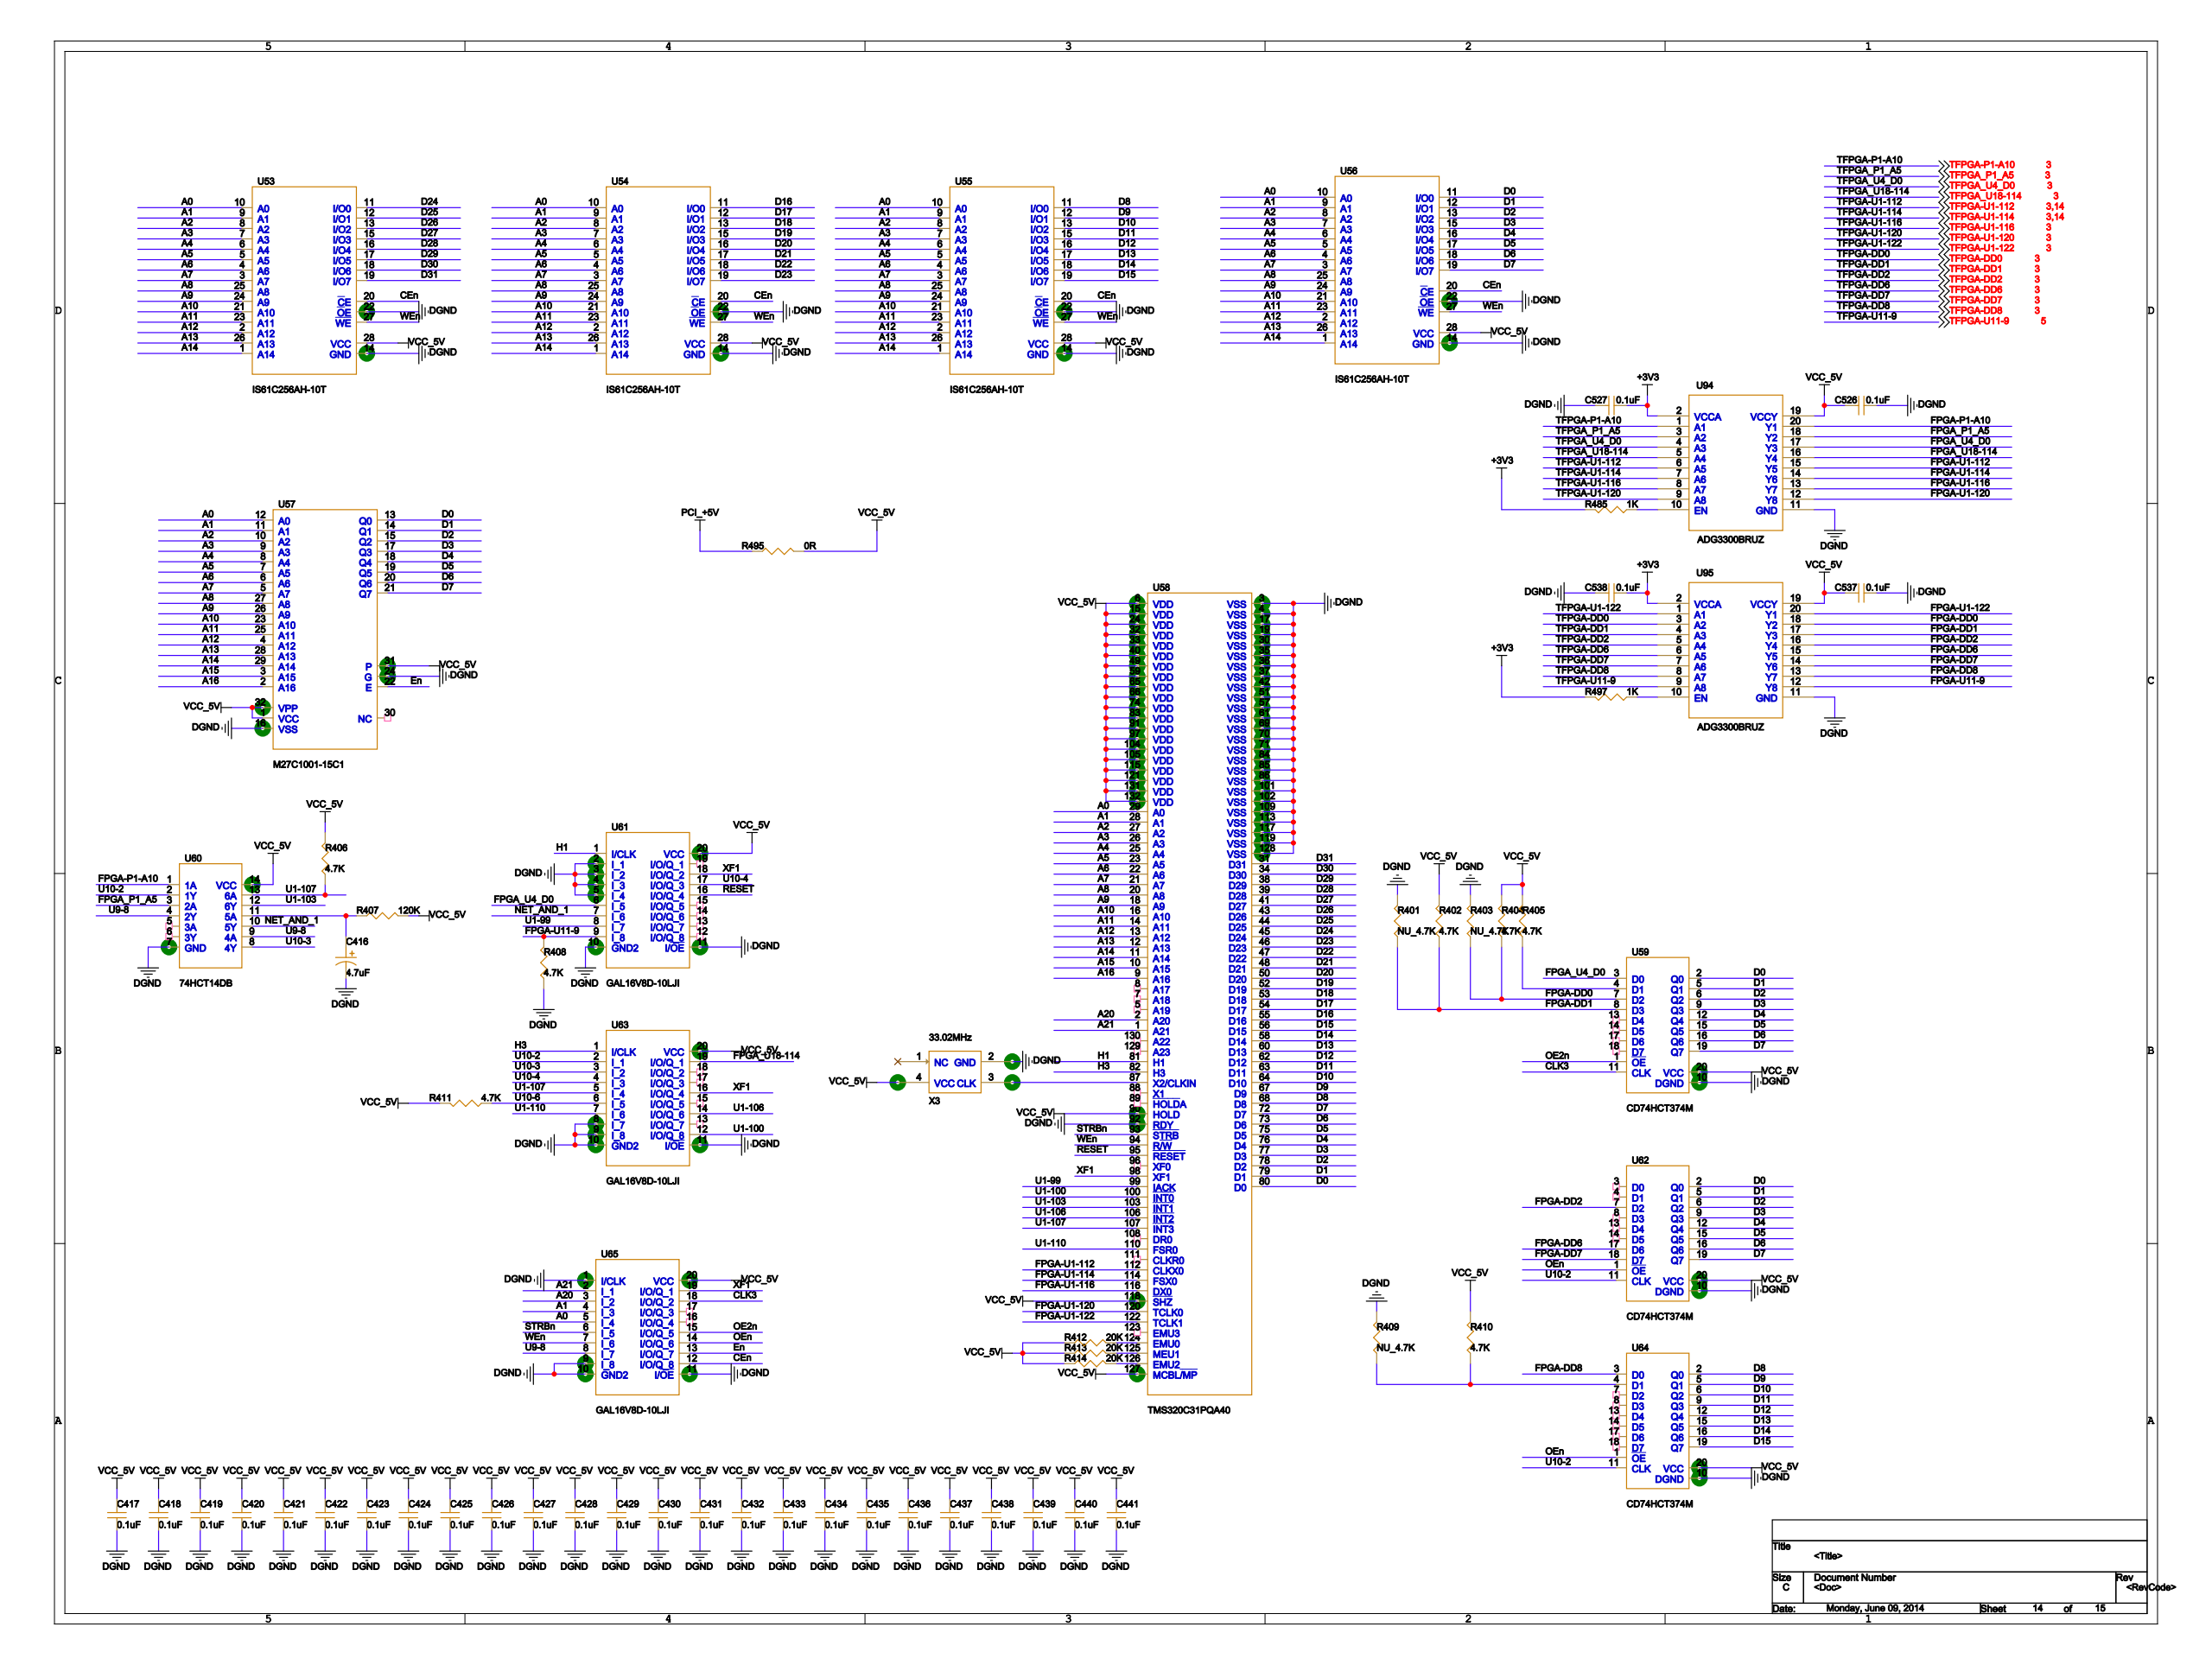Circuit board | Cadence Allegro | 669 parts | 806 nets | one sheet of the schematic
Parts on this sheet (reference | value | footprint):
C416 | 4.7uF | CP3216
C417 | 0.1uF | C0402
C418 | 0.1uF | C0402
C419 | 0.1uF | C0402
C420 | 0.1uF | C0402
C421 | 0.1uF | C0402
C422 | 0.1uF | C0402
C423 | 0.1uF | C0402
C424 | 0.1uF | C0402
C425 | 0.1uF | C0402
C426 | 0.1uF | C0402
C427 | 0.1uF | C0402
C428 | 0.1uF | C0402
C429 | 0.1uF | C0402
C430 | 0.1uF | C0402
C431 | 0.1uF | C0402
C432 | 0.1uF | C0402
C433 | 0.1uF | C0402
C434 | 0.1uF | C0402
C435 | 0.1uF | C0402
C436 | 0.1uF | C0402
C437 | 0.1uF | C0402
C438 | 0.1uF | C0402
C439 | 0.1uF | C0402
C440 | 0.1uF | C0402
C441 | 0.1uF | C0402
C526 | 0.1uF | C0402
C527 | 0.1uF | C0402
C537 | 0.1uF | C0402
C538 | 0.1uF | C0402
R401 | NU_4.7K | R0603
R402 | 4.7K | R0603
R403 | NU_4.7K | R0603
R404 | 4.7K | R0603
R405 | 4.7K | R0603
R406 | 4.7K | R0603
R407 | 120K | R0603
R408 | 4.7K | R0603
R409 | NU_4.7K | R0603
R410 | 4.7K | R0603
R411 | 4.7K | R0603
R412 | 20K | R0603
R413 | 20K | R0603
R414 | 20K | R0603
R485 | 1K | R0603
R495 | 0R | R1210
R497 | 1K | R0603
U53 | IS61C256AH-10T | TSOP28_0P55M_13P4X8M
U54 | IS61C256AH-10T | TSOP28_0P55M_13P4X8M
U55 | IS61C256AH-10T | TSOP28_0P55M_13P4X8M
U56 | IS61C256AH-10T | TSOP28_0P55M_13P4X8M
U57 | M27C1001-15C1 | PLCC32
U58 | TMS320C31PQA40 | QFP132_0P65M_28X28M
U59 | CD74HCT374M | SOIC20_1P27M_10X13M
U60 | 74HCT14DB | SSOP14
U61 | GAL16V8D-10LJI | PLCC20
U62 | CD74HCT374M | SOIC20_1P27M_10X13M
U63 | GAL16V8D-10LJI | PLCC20
U64 | CD74HCT374M | SOIC20_1P27M_10X13M
U65 | GAL16V8D-10LJI | PLCC20
U94 | ADG3300BRUZ | TSSOP20_0P65M_6P4X6P4M
U95 | ADG3300BRUZ | TSSOP20_0P65M_6P4X6P4M
X3 | 33.02MHz | OSC-SMD7050
Nets of these parts (net: part-pin ...):
DGND: C416-2 C417-1 C418-1 C419-1 C420-1 C421-1 C422-1 C423-1 C424-1 C425-1 C426-1 C427-1 C428-1 C429-1 C430-1 C431-1 C432-1 C433-1 C434-1 C435-1 C436-1 C437-1 C438-1 C439-1 C440-1 C441-1 C526-1 C527-2 C537-1 C538-2 R401-2 R403-2 R408-1 R409-2 U59-10 U60-7 U61-2 U61-3 U61-4 U61-5 U61-10 U61-11 U62-10 U63-8 U63-9 U63-10 U63-11 U64-10 U65-1 U65-9 U65-10 U65-11 U94-11 U95-11 X3-2 U53-14 U53-22 U54-14 U54-22 U55-14 U55-22 U56-14 U56-22 U57-16 U57-24 U58-3 U58-4 U58-17 U58-19 U58-30 U58-35 U58-36 U58-37 U58-42 U58-51 U58-57 U58-61 U58-69 U58-70 U58-71 U58-84 U58-85 U58-86 U58-92 U58-101 U58-102 U58-109 U58-113 U58-117 U58-119 U58-128
+3V3: C527-1 C538-1 R485-2 R497-2 U94-2 U95-2
TFPGA-DD6: U95-6
TFPGA_U4_D0: U94-4
TFPGA_U18-114: U94-5
TFPGA-U1-112: U94-6
TFPGA-DD0: U95-3
TFPGA-DD8: U95-8
TFPGA-U1-120: U94-9
TFPGA-U1-122: U95-1
TFPGA-U1-114: U94-7
TFPGA-U1-116: U94-8
TFPGA_P1_A5: U94-3
TFPGA-DD2: U95-5
TFPGA-P1-A10: U94-1
TFPGA-DD7: U95-7
TFPGA-U11-9: U95-9
TFPGA-DD1: U95-4
A0: U65-5 U53-10 U54-10 U55-10 U56-10 U57-12 U58-29
A1: U65-4 U53-9 U54-9 U55-9 U56-9 U57-11 U58-28
A10: U53-21 U54-21 U55-21 U56-21 U57-23 U58-16
A11: U53-23 U54-23 U55-23 U56-23 U57-25 U58-14
A12: U53-2 U54-2 U55-2 U56-2 U57-4 U58-13
A13: U53-26 U54-26 U55-26 U56-26 U57-28 U58-12
A14: U53-1 U54-1 U55-1 U56-1 U57-29 U58-11
A2: U53-8 U54-8 U55-8 U56-8 U57-10 U58-27
A3: U53-7 U54-7 U55-7 U56-7 U57-9 U58-26
A4: U53-6 U54-6 U55-6 U56-6 U57-8 U58-25
A5: U53-5 U54-5 U55-5 U56-5 U57-7 U58-23
A6: U53-4 U54-4 U55-4 U56-4 U57-6 U58-22
A7: U53-3 U54-3 U55-3 U56-3 U57-5 U58-21
A8: U53-25 U54-25 U55-25 U56-25 U57-27 U58-20
A9: U53-24 U54-24 U55-24 U56-24 U57-26 U58-18
D24: U53-11 U58-45
D25: U53-12 U58-44
D26: U53-13 U58-43
D27: U53-15 U58-41
D28: U53-16 U58-39
D29: U53-17 U58-38
D30: U53-18 U58-34
D31: U53-19 U58-31
VCC_5V: C417-2 C418-2 C419-2 C420-2 C421-2 C422-2 C423-2 C424-2 C425-2 C426-2 C427-2 C428-2 C429-2 C430-2 C431-2 C432-2 C433-2 C434-2 C435-2 C436-2 C437-2 C438-2 C439-2 C440-2 C441-2 C526-2 C537-2 R402-2 R404-2 R405-2 R406-2 R407-2 R410-2 R411-2 R412-1 R413-1 R414-1 R495-2 U59-20 U60-14 U61-20 U62-20 U63-20 U64-20 U65-20 U94-19 U95-19 X3-4 U53-28 U54-28 U55-28 U56-28 U57-1 U57-31 U57-32 U58-6 U58-15 U58-24 U58-32 U58-33 U58-40 U58-49 U58-59 U58-65 U58-66 U58-74 U58-83 U58-90 U58-91 U58-97 U58-104 U58-105 U58-115 U58-118 U58-121 U58-127 U58-131 U58-132
CEN: U65-12 U53-20 U54-20 U55-20 U56-20
WEN: U65-7 U53-27 U54-27 U55-27 U56-27 U58-94
D16: U54-11 U58-55
D17: U54-12 U58-54
D18: U54-13 U58-53
D19: U54-15 U58-52
D20: U54-16 U58-50
D21: U54-17 U58-48
D22: U54-18 U58-47
D23: U54-19 U58-46
D8: U64-2 U55-11 U58-68
D9: U64-5 U55-12 U58-67
D10: U64-6 U55-13 U58-64
D11: U64-9 U55-15 U58-63
D12: U64-12 U55-16 U58-62
D13: U64-15 U55-17 U58-60
D14: U64-16 U55-18 U58-58
D15: U64-19 U55-19 U58-56
D0: U59-2 U62-2 U56-11 U57-13 U58-80
D1: U59-5 U62-5 U56-12 U57-14 U58-79
D2: U59-6 U62-6 U56-13 U57-15 U58-78
D3: U59-9 U62-9 U56-15 U57-17 U58-77
D4: U59-12 U62-12 U56-16 U57-18 U58-76
D5: U59-15 U62-15 U56-17 U57-19 U58-75
D6: U59-16 U62-16 U56-18 U57-20 U58-73
D7: U59-19 U62-19 U56-19 U57-21 U58-72
A15: U57-3 U58-10
A16: U57-2 U58-9
EN: U65-13 U57-22
A20: U65-3 U58-2
A21: U65-2 U58-1
FPGA-U1-112: U94-15 U58-112
FPGA-U1-116: U94-13 U58-116
N16294046: R412-2 U58-124
N16294054: R414-2 U58-126
U1-110: U63-7 U58-110
FPGA-U1-114: U94-14 U58-114
H1: U61-1 U58-81
H3: U63-1 U58-82
U1-99: U61-8 U58-99
N16294050: R413-2 U58-125
FPGA-U1-120: U94-12 U58-120
FPGA-U1-122: U95-20 U58-122
N16295478: X3-3 U58-87
XF1: U61-18 U63-16 U65-19 U58-98
U1-100: U63-12 U58-100
U1-103: U60-12 U58-103
U1-106: U63-14 U58-106
U1-107: R406-1 U60-13 U63-5 U58-107
RESET: U61-16 U58-95
STRBN: U65-6 U58-93
CLK3: U59-11 U65-18
FPGA_U4_D0: U59-3 U61-6 U94-17
N16297271: R405-1 U59-4
FPGA-DD0: R403-1 R404-1 U59-7 U95-18
FPGA-DD1: R401-1 R402-1 U59-8 U95-17
OE2N: U59-1 U65-15
U10-2: U60-2 U62-11 U63-2 U64-11
FPGA-DD2: U62-7 U95-16
FPGA-DD6: U62-17 U95-15
FPGA-DD7: U62-18 U95-14
OEN: U62-1 U64-1 U65-14
FPGA-DD8: U64-3 U95-13
N16301632: R409-1 R410-1 U64-4
FPGA-P1-A10: U60-1 U94-20
FPGA_P1_A5: U60-3 U94-18
U9-8: U60-4 U60-9 U65-8
U10-3: U60-8 U63-3
N16302998: C416-1 R407-1 U60-11
NET_AND_1: U60-10 U61-7
U10-4: U61-17 U63-4
FPGA-U11-9: R408-2 U61-9 U95-12
FPGA_U18-114: U63-19 U94-16
U10-6: R411-1 U63-6
N61236976: R485-1 U94-10
N61237895: R497-1 U95-10
PCI_+5V: R495-1